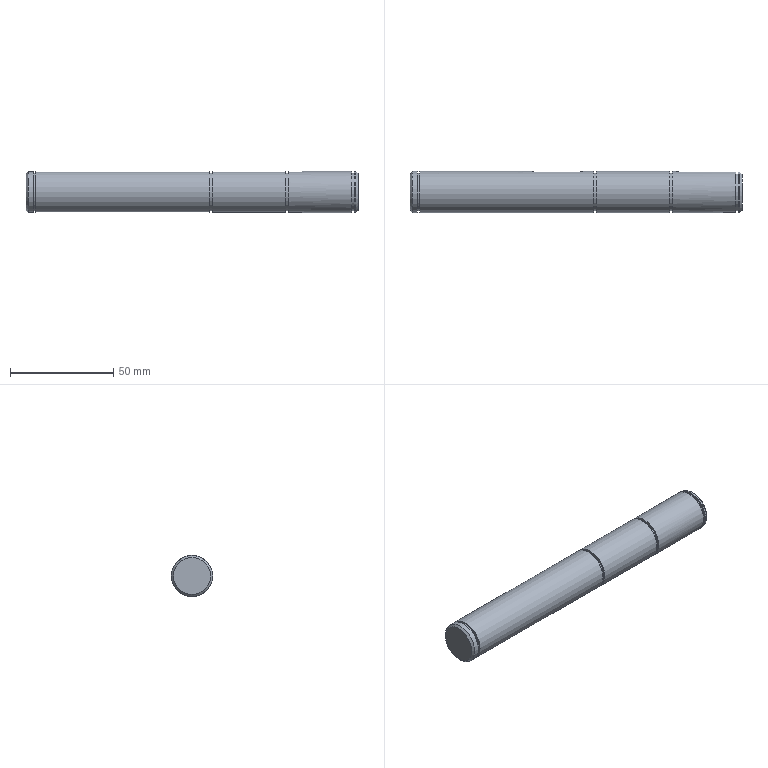Part | STEP file | Shaft1 | 1 solid | 30 faces | box 161 x 20 x 20 mm | volume 49512 mm3 | plane 16 | cylinder 12 | cone 2 | commonest cylinder face diameters 20 x5 18.35 x4 6 x3